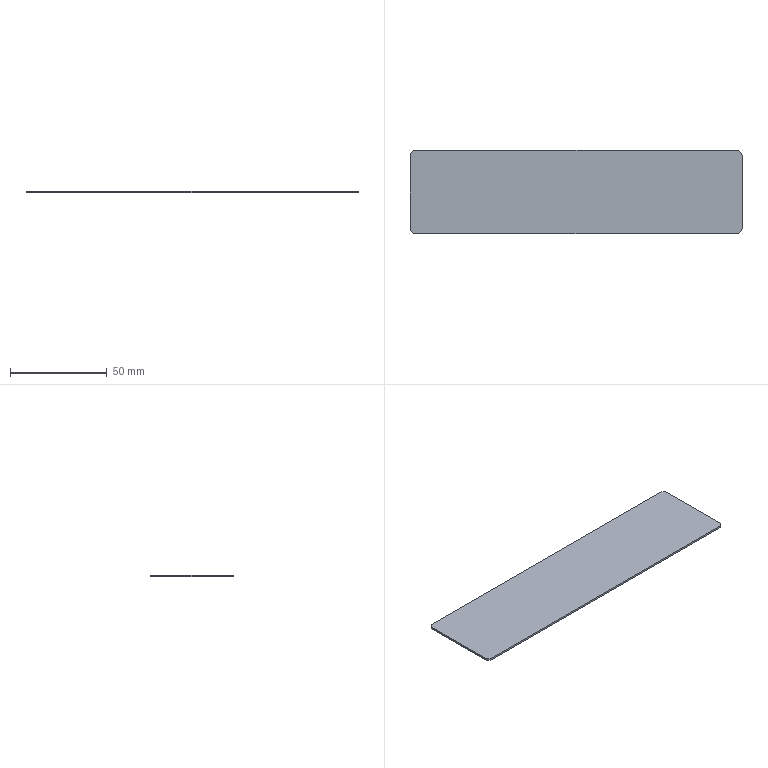Part | SolidWorks | features MirrorStock 1 | 1 solid | 10 faces | box 172 x 43.4 x 1 mm | volume 7457 mm3 | plane 6 | cylinder 4 | commonest cylinder face diameters 6 x4
STEP:
#1=CARTESIAN_POINT('',(83.,-14.4,-65.));
#2=VERTEX_POINT('',#1);
#3=CARTESIAN_POINT('',(86.,-11.4,-65.));
#4=VERTEX_POINT('',#3);
#5=CARTESIAN_POINT('',(83.,-11.4,-65.));
#6=DIRECTION('',(0.,0.,1.));
#7=DIRECTION('',(1.,0.,0.));
#8=AXIS2_PLACEMENT_3D('',#5,#6,#7);
#9=CIRCLE('',#8,3.);
#10=EDGE_CURVE('',#2,#4,#9,.T.);
#11=ORIENTED_EDGE('',*,*,#10,.F.);
#12=CARTESIAN_POINT('',(-83.,-14.4,-65.));
#13=VERTEX_POINT('',#12);
#14=CARTESIAN_POINT('',(0.,-14.4,-65.));
#15=DIRECTION('',(-1.,0.,0.));
#16=VECTOR('',#15,1000.);
#17=LINE('',#14,#16);
#18=EDGE_CURVE('',#2,#13,#17,.T.);
#19=ORIENTED_EDGE('',*,*,#18,.T.);
#20=CARTESIAN_POINT('',(-86.,-11.4,-65.));
#21=VERTEX_POINT('',#20);
#22=CARTESIAN_POINT('',(-83.,-11.4,-65.));
#23=DIRECTION('',(0.,0.,1.));
#24=DIRECTION('',(1.,0.,0.));
#25=AXIS2_PLACEMENT_3D('',#22,#23,#24);
#26=CIRCLE('',#25,3.);
#27=EDGE_CURVE('',#21,#13,#26,.T.);
#28=ORIENTED_EDGE('',*,*,#27,.F.);
#29=CARTESIAN_POINT('',(-86.,26.,-65.));
#30=VERTEX_POINT('',#29);
#31=CARTESIAN_POINT('',(-86.,7.3,-65.));
#32=DIRECTION('',(0.,1.,0.));
#33=VECTOR('',#32,1000.);
#34=LINE('',#31,#33);
#35=EDGE_CURVE('',#21,#30,#34,.T.);
#36=ORIENTED_EDGE('',*,*,#35,.T.);
#37=CARTESIAN_POINT('',(-83.,29.,-65.));
#38=VERTEX_POINT('',#37);
#39=CARTESIAN_POINT('',(-83.,26.,-65.));
#40=DIRECTION('',(0.,0.,1.));
#41=DIRECTION('',(1.,0.,0.));
#42=AXIS2_PLACEMENT_3D('',#39,#40,#41);
#43=CIRCLE('',#42,3.);
#44=EDGE_CURVE('',#38,#30,#43,.T.);
#45=ORIENTED_EDGE('',*,*,#44,.F.);
#46=CARTESIAN_POINT('',(83.,29.,-65.));
#47=VERTEX_POINT('',#46);
#48=CARTESIAN_POINT('',(0.,29.,-65.));
#49=DIRECTION('',(1.,0.,0.));
#50=VECTOR('',#49,1000.);
#51=LINE('',#48,#50);
#52=EDGE_CURVE('',#38,#47,#51,.T.);
#53=ORIENTED_EDGE('',*,*,#52,.T.);
#54=CARTESIAN_POINT('',(86.,26.,-65.));
#55=VERTEX_POINT('',#54);
#56=CARTESIAN_POINT('',(83.,26.,-65.));
#57=DIRECTION('',(0.,0.,1.));
#58=DIRECTION('',(1.,0.,0.));
#59=AXIS2_PLACEMENT_3D('',#56,#57,#58);
#60=CIRCLE('',#59,3.);
#61=EDGE_CURVE('',#55,#47,#60,.T.);
#62=ORIENTED_EDGE('',*,*,#61,.F.);
#63=CARTESIAN_POINT('',(86.,7.3,-65.));
#64=DIRECTION('',(0.,-1.,0.));
#65=VECTOR('',#64,1000.);
#66=LINE('',#63,#65);
#67=EDGE_CURVE('',#55,#4,#66,.T.);
#68=ORIENTED_EDGE('',*,*,#67,.T.);
#69=EDGE_LOOP('',(#11,#19,#28,#36,#45,#53,#62,#68));
#70=FACE_OUTER_BOUND('',#69,.T.);
#71=CARTESIAN_POINT('',(-89.44,29.868,-65.));
#72=DIRECTION('',(0.,0.,-1.));
#73=DIRECTION('',(0.,-1.,0.));
#74=AXIS2_PLACEMENT_3D('',#71,#72,#73);
#75=PLANE('',#74);
#76=ADVANCED_FACE('',(#70),#75,.T.);
#77=ORIENTED_EDGE('',*,*,#61,.T.);
#78=CARTESIAN_POINT('',(83.,29.,-64.));
#79=VERTEX_POINT('',#78);
#80=CARTESIAN_POINT('',(83.,29.,-64.5));
#81=DIRECTION('',(0.,0.,1.));
#82=VECTOR('',#81,1000.);
#83=LINE('',#80,#82);
#84=EDGE_CURVE('',#47,#79,#83,.T.);
#85=ORIENTED_EDGE('',*,*,#84,.T.);
#86=CARTESIAN_POINT('',(86.,26.,-64.));
#87=VERTEX_POINT('',#86);
#88=CARTESIAN_POINT('',(83.,26.,-64.));
#89=DIRECTION('',(0.,0.,1.));
#90=DIRECTION('',(1.,0.,0.));
#91=AXIS2_PLACEMENT_3D('',#88,#89,#90);
#92=CIRCLE('',#91,3.);
#93=EDGE_CURVE('',#87,#79,#92,.T.);
#94=ORIENTED_EDGE('',*,*,#93,.F.);
#95=CARTESIAN_POINT('',(86.,26.,-64.5));
#96=DIRECTION('',(0.,0.,-1.));
#97=VECTOR('',#96,1000.);
#98=LINE('',#95,#97);
#99=EDGE_CURVE('',#87,#55,#98,.T.);
#100=ORIENTED_EDGE('',*,*,#99,.T.);
#101=EDGE_LOOP('',(#77,#85,#94,#100));
#102=FACE_OUTER_BOUND('',#101,.T.);
#103=CARTESIAN_POINT('',(83.,26.,-64.));
#104=DIRECTION('',(0.,0.,-1.));
#105=DIRECTION('',(1.,0.,0.));
#106=AXIS2_PLACEMENT_3D('',#103,#104,#105);
#107=CYLINDRICAL_SURFACE('',#106,3.);
#108=ADVANCED_FACE('',(#102),#107,.T.);
#109=ORIENTED_EDGE('',*,*,#52,.F.);
#110=CARTESIAN_POINT('',(-83.,29.,-64.));
#111=VERTEX_POINT('',#110);
#112=CARTESIAN_POINT('',(-83.,29.,-64.5));
#113=DIRECTION('',(0.,0.,-1.));
#114=VECTOR('',#113,1000.);
#115=LINE('',#112,#114);
#116=EDGE_CURVE('',#111,#38,#115,.T.);
#117=ORIENTED_EDGE('',*,*,#116,.F.);
#118=CARTESIAN_POINT('',(0.,29.,-64.));
#119=DIRECTION('',(-1.,0.,0.));
#120=VECTOR('',#119,1000.);
#121=LINE('',#118,#120);
#122=EDGE_CURVE('',#79,#111,#121,.T.);
#123=ORIENTED_EDGE('',*,*,#122,.F.);
#124=ORIENTED_EDGE('',*,*,#84,.F.);
#125=EDGE_LOOP('',(#109,#117,#123,#124));
#126=FACE_OUTER_BOUND('',#125,.T.);
#127=CARTESIAN_POINT('',(86.32,29.,-63.787));
#128=DIRECTION('',(0.,1.,0.));
#129=DIRECTION('',(-1.,0.,0.));
#130=AXIS2_PLACEMENT_3D('',#127,#128,#129);
#131=PLANE('',#130);
#132=ADVANCED_FACE('',(#126),#131,.T.);
#133=ORIENTED_EDGE('',*,*,#44,.T.);
#134=CARTESIAN_POINT('',(-86.,26.,-64.));
#135=VERTEX_POINT('',#134);
#136=CARTESIAN_POINT('',(-86.,26.,-64.5));
#137=DIRECTION('',(0.,0.,1.));
#138=VECTOR('',#137,1000.);
#139=LINE('',#136,#138);
#140=EDGE_CURVE('',#30,#135,#139,.T.);
#141=ORIENTED_EDGE('',*,*,#140,.T.);
#142=CARTESIAN_POINT('',(-83.,26.,-64.));
#143=DIRECTION('',(0.,0.,1.));
#144=DIRECTION('',(1.,0.,0.));
#145=AXIS2_PLACEMENT_3D('',#142,#143,#144);
#146=CIRCLE('',#145,3.);
#147=EDGE_CURVE('',#111,#135,#146,.T.);
#148=ORIENTED_EDGE('',*,*,#147,.F.);
#149=ORIENTED_EDGE('',*,*,#116,.T.);
#150=EDGE_LOOP('',(#133,#141,#148,#149));
#151=FACE_OUTER_BOUND('',#150,.T.);
#152=CARTESIAN_POINT('',(-83.,26.,-64.));
#153=DIRECTION('',(0.,0.,-1.));
#154=DIRECTION('',(1.,0.,0.));
#155=AXIS2_PLACEMENT_3D('',#152,#153,#154);
#156=CYLINDRICAL_SURFACE('',#155,3.);
#157=ADVANCED_FACE('',(#151),#156,.T.);
#158=ORIENTED_EDGE('',*,*,#35,.F.);
#159=CARTESIAN_POINT('',(-86.,-11.4,-64.));
#160=VERTEX_POINT('',#159);
#161=CARTESIAN_POINT('',(-86.,-11.4,-64.5));
#162=DIRECTION('',(0.,0.,-1.));
#163=VECTOR('',#162,1000.);
#164=LINE('',#161,#163);
#165=EDGE_CURVE('',#160,#21,#164,.T.);
#166=ORIENTED_EDGE('',*,*,#165,.F.);
#167=CARTESIAN_POINT('',(-86.,7.3,-64.));
#168=DIRECTION('',(0.,-1.,0.));
#169=VECTOR('',#168,1000.);
#170=LINE('',#167,#169);
#171=EDGE_CURVE('',#135,#160,#170,.T.);
#172=ORIENTED_EDGE('',*,*,#171,.F.);
#173=ORIENTED_EDGE('',*,*,#140,.F.);
#174=EDGE_LOOP('',(#158,#166,#172,#173));
#175=FACE_OUTER_BOUND('',#174,.T.);
#176=CARTESIAN_POINT('',(-86.,26.748,-63.787));
#177=DIRECTION('',(-1.,0.,0.));
#178=DIRECTION('',(0.,-1.,0.));
#179=AXIS2_PLACEMENT_3D('',#176,#177,#178);
#180=PLANE('',#179);
#181=ADVANCED_FACE('',(#175),#180,.T.);
#182=ORIENTED_EDGE('',*,*,#27,.T.);
#183=CARTESIAN_POINT('',(-83.,-14.4,-64.));
#184=VERTEX_POINT('',#183);
#185=CARTESIAN_POINT('',(-83.,-14.4,-64.5));
#186=DIRECTION('',(0.,0.,1.));
#187=VECTOR('',#186,1000.);
#188=LINE('',#185,#187);
#189=EDGE_CURVE('',#13,#184,#188,.T.);
#190=ORIENTED_EDGE('',*,*,#189,.T.);
#191=CARTESIAN_POINT('',(-83.,-11.4,-64.));
#192=DIRECTION('',(0.,0.,1.));
#193=DIRECTION('',(1.,0.,0.));
#194=AXIS2_PLACEMENT_3D('',#191,#192,#193);
#195=CIRCLE('',#194,3.);
#196=EDGE_CURVE('',#160,#184,#195,.T.);
#197=ORIENTED_EDGE('',*,*,#196,.F.);
#198=ORIENTED_EDGE('',*,*,#165,.T.);
#199=EDGE_LOOP('',(#182,#190,#197,#198));
#200=FACE_OUTER_BOUND('',#199,.T.);
#201=CARTESIAN_POINT('',(-83.,-11.4,-64.));
#202=DIRECTION('',(0.,0.,-1.));
#203=DIRECTION('',(1.,0.,0.));
#204=AXIS2_PLACEMENT_3D('',#201,#202,#203);
#205=CYLINDRICAL_SURFACE('',#204,3.);
#206=ADVANCED_FACE('',(#200),#205,.T.);
#207=ORIENTED_EDGE('',*,*,#18,.F.);
#208=CARTESIAN_POINT('',(83.,-14.4,-64.));
#209=VERTEX_POINT('',#208);
#210=CARTESIAN_POINT('',(83.,-14.4,-64.5));
#211=DIRECTION('',(0.,0.,-1.));
#212=VECTOR('',#211,1000.);
#213=LINE('',#210,#212);
#214=EDGE_CURVE('',#209,#2,#213,.T.);
#215=ORIENTED_EDGE('',*,*,#214,.F.);
#216=CARTESIAN_POINT('',(0.,-14.4,-64.));
#217=DIRECTION('',(1.,0.,0.));
#218=VECTOR('',#217,1000.);
#219=LINE('',#216,#218);
#220=EDGE_CURVE('',#184,#209,#219,.T.);
#221=ORIENTED_EDGE('',*,*,#220,.F.);
#222=ORIENTED_EDGE('',*,*,#189,.F.);
#223=EDGE_LOOP('',(#207,#215,#221,#222));
#224=FACE_OUTER_BOUND('',#223,.T.);
#225=CARTESIAN_POINT('',(-86.32,-14.4,-63.787));
#226=DIRECTION('',(0.,-1.,0.));
#227=DIRECTION('',(1.,0.,0.));
#228=AXIS2_PLACEMENT_3D('',#225,#226,#227);
#229=PLANE('',#228);
#230=ADVANCED_FACE('',(#224),#229,.T.);
#231=ORIENTED_EDGE('',*,*,#10,.T.);
#232=CARTESIAN_POINT('',(86.,-11.4,-64.));
#233=VERTEX_POINT('',#232);
#234=CARTESIAN_POINT('',(86.,-11.4,-64.5));
#235=DIRECTION('',(0.,0.,1.));
#236=VECTOR('',#235,1000.);
#237=LINE('',#234,#236);
#238=EDGE_CURVE('',#4,#233,#237,.T.);
#239=ORIENTED_EDGE('',*,*,#238,.T.);
#240=CARTESIAN_POINT('',(83.,-11.4,-64.));
#241=DIRECTION('',(0.,0.,1.));
#242=DIRECTION('',(1.,0.,0.));
#243=AXIS2_PLACEMENT_3D('',#240,#241,#242);
#244=CIRCLE('',#243,3.);
#245=EDGE_CURVE('',#209,#233,#244,.T.);
#246=ORIENTED_EDGE('',*,*,#245,.F.);
#247=ORIENTED_EDGE('',*,*,#214,.T.);
#248=EDGE_LOOP('',(#231,#239,#246,#247));
#249=FACE_OUTER_BOUND('',#248,.T.);
#250=CARTESIAN_POINT('',(83.,-11.4,-64.));
#251=DIRECTION('',(0.,0.,-1.));
#252=DIRECTION('',(1.,0.,0.));
#253=AXIS2_PLACEMENT_3D('',#250,#251,#252);
#254=CYLINDRICAL_SURFACE('',#253,3.);
#255=ADVANCED_FACE('',(#249),#254,.T.);
#256=ORIENTED_EDGE('',*,*,#67,.F.);
#257=ORIENTED_EDGE('',*,*,#99,.F.);
#258=CARTESIAN_POINT('',(86.,7.3,-64.));
#259=DIRECTION('',(0.,1.,0.));
#260=VECTOR('',#259,1000.);
#261=LINE('',#258,#260);
#262=EDGE_CURVE('',#233,#87,#261,.T.);
#263=ORIENTED_EDGE('',*,*,#262,.F.);
#264=ORIENTED_EDGE('',*,*,#238,.F.);
#265=EDGE_LOOP('',(#256,#257,#263,#264));
#266=FACE_OUTER_BOUND('',#265,.T.);
#267=CARTESIAN_POINT('',(86.,-12.148,-63.787));
#268=DIRECTION('',(1.,0.,0.));
#269=DIRECTION('',(0.,1.,0.));
#270=AXIS2_PLACEMENT_3D('',#267,#268,#269);
#271=PLANE('',#270);
#272=ADVANCED_FACE('',(#266),#271,.T.);
#273=ORIENTED_EDGE('',*,*,#245,.T.);
#274=ORIENTED_EDGE('',*,*,#262,.T.);
#275=ORIENTED_EDGE('',*,*,#93,.T.);
#276=ORIENTED_EDGE('',*,*,#122,.T.);
#277=ORIENTED_EDGE('',*,*,#147,.T.);
#278=ORIENTED_EDGE('',*,*,#171,.T.);
#279=ORIENTED_EDGE('',*,*,#196,.T.);
#280=ORIENTED_EDGE('',*,*,#220,.T.);
#281=EDGE_LOOP('',(#273,#274,#275,#276,#277,#278,#279,#280));
#282=FACE_OUTER_BOUND('',#281,.T.);
#283=CARTESIAN_POINT('',(-89.44,29.868,-64.));
#284=DIRECTION('',(0.,0.,-1.));
#285=DIRECTION('',(0.,-1.,0.));
#286=AXIS2_PLACEMENT_3D('',#283,#284,#285);
#287=PLANE('',#286);
#288=ADVANCED_FACE('',(#282),#287,.F.);
#289=CLOSED_SHELL('',(#76,#108,#132,#157,#181,#206,#230,#255,#272,#288));
#290=MANIFOLD_SOLID_BREP('',#289);
#291=CARTESIAN_POINT('',(0.,0.,0.));
#292=DIRECTION('',(0.,0.,1.));
#293=DIRECTION('',(1.,0.,0.));
#294=AXIS2_PLACEMENT_3D('',#291,#292,#293);
#295=(LENGTH_UNIT()NAMED_UNIT(*)SI_UNIT(.MILLI.,.METRE.));
#296=UNCERTAINTY_MEASURE_WITH_UNIT(LENGTH_MEASURE(0.00001),#295,'','');
#297=(NAMED_UNIT(*)PLANE_ANGLE_UNIT()SI_UNIT($,.RADIAN.));
#298=(NAMED_UNIT(*)SI_UNIT($,.STERADIAN.)SOLID_ANGLE_UNIT());
#299=(GEOMETRIC_REPRESENTATION_CONTEXT(3)GLOBAL_UNCERTAINTY_ASSIGNED_CONTEXT((#296))GLOBAL_UNIT_ASSIGNED_CONTEXT((#295,#297,#298))REPRESENTATION_CONTEXT('',''));
#300=ADVANCED_BREP_SHAPE_REPRESENTATION('',(#290,#294),#299);